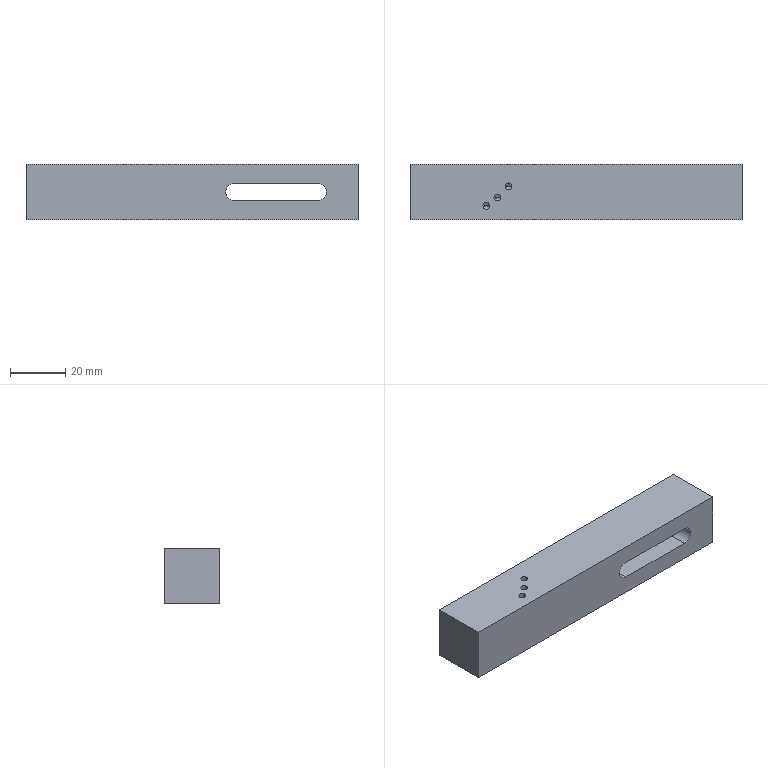Part | SolidWorks | features ICE 5, HoleWzd 2, Extrusion 1 | 1 solid | 22 faces | box 120 x 20 x 20 mm | volume 43402 mm3 | cylinder 8 | plane 8 | cone 6 | commonest cylinder face diameters 2.5 x6 6.4 x2
STEP:
#1=CARTESIAN_POINT('',(-64.65,108.,2.5));
#2=VERTEX_POINT('',#1);
#3=CARTESIAN_POINT('',(-62.15,108.,2.5));
#4=VERTEX_POINT('',#3);
#5=CARTESIAN_POINT('',(-63.4,108.,2.5));
#6=DIRECTION('',(0.,0.,1.));
#7=DIRECTION('',(1.,0.,0.));
#8=AXIS2_PLACEMENT_3D('',#5,#6,#7);
#9=CIRCLE('',#8,1.25);
#10=EDGE_CURVE('',#2,#4,#9,.T.);
#11=ORIENTED_EDGE('',*,*,#10,.F.);
#12=CARTESIAN_POINT('',(-64.65,108.,10.));
#13=VERTEX_POINT('',#12);
#14=CARTESIAN_POINT('',(-64.65,108.,10.));
#15=DIRECTION('',(0.,0.,1.));
#16=VECTOR('',#15,1000.);
#17=LINE('',#14,#16);
#18=EDGE_CURVE('',#2,#13,#17,.T.);
#19=ORIENTED_EDGE('',*,*,#18,.T.);
#20=CARTESIAN_POINT('',(-62.15,108.,10.));
#21=VERTEX_POINT('',#20);
#22=CARTESIAN_POINT('',(-63.4,108.,10.));
#23=DIRECTION('',(0.,0.,1.));
#24=DIRECTION('',(1.,0.,0.));
#25=AXIS2_PLACEMENT_3D('',#22,#23,#24);
#26=CIRCLE('',#25,1.25);
#27=EDGE_CURVE('',#13,#21,#26,.T.);
#28=ORIENTED_EDGE('',*,*,#27,.T.);
#29=CARTESIAN_POINT('',(-62.15,108.,10.));
#30=DIRECTION('',(0.,0.,1.));
#31=VECTOR('',#30,1000.);
#32=LINE('',#29,#31);
#33=EDGE_CURVE('',#4,#21,#32,.T.);
#34=ORIENTED_EDGE('',*,*,#33,.F.);
#35=EDGE_LOOP('',(#11,#19,#28,#34));
#36=FACE_OUTER_BOUND('',#35,.T.);
#37=CARTESIAN_POINT('',(-63.4,108.,10.));
#38=DIRECTION('',(0.,0.,1.));
#39=DIRECTION('',(1.,0.,0.));
#40=AXIS2_PLACEMENT_3D('',#37,#38,#39);
#41=CYLINDRICAL_SURFACE('',#40,1.25);
#42=ADVANCED_FACE('',(#36),#41,.F.);
#43=CARTESIAN_POINT('',(-63.4,108.,1.749));
#44=VERTEX_POINT('',#43);
#45=CARTESIAN_POINT('',(-62.15,108.,2.5));
#46=DIRECTION('',(0.8572,0.,0.515));
#47=VECTOR('',#46,1000.);
#48=LINE('',#45,#47);
#49=EDGE_CURVE('',#44,#4,#48,.T.);
#50=ORIENTED_EDGE('',*,*,#49,.F.);
#51=CARTESIAN_POINT('',(-64.65,108.,2.5));
#52=DIRECTION('',(-0.8572,0.,0.515));
#53=VECTOR('',#52,1000.);
#54=LINE('',#51,#53);
#55=EDGE_CURVE('',#44,#2,#54,.T.);
#56=ORIENTED_EDGE('',*,*,#55,.T.);
#57=ORIENTED_EDGE('',*,*,#10,.T.);
#58=EDGE_LOOP('',(#50,#56,#57));
#59=FACE_OUTER_BOUND('',#58,.T.);
#60=CARTESIAN_POINT('',(-63.4,108.,2.5));
#61=DIRECTION('',(0.,0.,1.));
#62=DIRECTION('',(1.,0.,0.));
#63=AXIS2_PLACEMENT_3D('',#60,#61,#62);
#64=CONICAL_SURFACE('',#63,1.25,1.03);
#65=ADVANCED_FACE('',(#59),#64,.F.);
#66=CARTESIAN_POINT('',(-60.65,112.,2.5));
#67=VERTEX_POINT('',#66);
#68=CARTESIAN_POINT('',(-58.15,112.,2.5));
#69=VERTEX_POINT('',#68);
#70=CARTESIAN_POINT('',(-59.4,112.,2.5));
#71=DIRECTION('',(0.,0.,1.));
#72=DIRECTION('',(1.,0.,0.));
#73=AXIS2_PLACEMENT_3D('',#70,#71,#72);
#74=CIRCLE('',#73,1.25);
#75=EDGE_CURVE('',#67,#69,#74,.T.);
#76=ORIENTED_EDGE('',*,*,#75,.F.);
#77=CARTESIAN_POINT('',(-60.65,112.,10.));
#78=VERTEX_POINT('',#77);
#79=CARTESIAN_POINT('',(-60.65,112.,10.));
#80=DIRECTION('',(0.,0.,1.));
#81=VECTOR('',#80,1000.);
#82=LINE('',#79,#81);
#83=EDGE_CURVE('',#67,#78,#82,.T.);
#84=ORIENTED_EDGE('',*,*,#83,.T.);
#85=CARTESIAN_POINT('',(-58.15,112.,10.));
#86=VERTEX_POINT('',#85);
#87=CARTESIAN_POINT('',(-59.4,112.,10.));
#88=DIRECTION('',(0.,0.,1.));
#89=DIRECTION('',(1.,0.,0.));
#90=AXIS2_PLACEMENT_3D('',#87,#88,#89);
#91=CIRCLE('',#90,1.25);
#92=EDGE_CURVE('',#78,#86,#91,.T.);
#93=ORIENTED_EDGE('',*,*,#92,.T.);
#94=CARTESIAN_POINT('',(-58.15,112.,10.));
#95=DIRECTION('',(0.,0.,1.));
#96=VECTOR('',#95,1000.);
#97=LINE('',#94,#96);
#98=EDGE_CURVE('',#69,#86,#97,.T.);
#99=ORIENTED_EDGE('',*,*,#98,.F.);
#100=EDGE_LOOP('',(#76,#84,#93,#99));
#101=FACE_OUTER_BOUND('',#100,.T.);
#102=CARTESIAN_POINT('',(-59.4,112.,10.));
#103=DIRECTION('',(0.,0.,1.));
#104=DIRECTION('',(1.,0.,0.));
#105=AXIS2_PLACEMENT_3D('',#102,#103,#104);
#106=CYLINDRICAL_SURFACE('',#105,1.25);
#107=ADVANCED_FACE('',(#101),#106,.F.);
#108=CARTESIAN_POINT('',(-59.4,112.,1.749));
#109=VERTEX_POINT('',#108);
#110=CARTESIAN_POINT('',(-58.15,112.,2.5));
#111=DIRECTION('',(0.8572,0.,0.515));
#112=VECTOR('',#111,1000.);
#113=LINE('',#110,#112);
#114=EDGE_CURVE('',#109,#69,#113,.T.);
#115=ORIENTED_EDGE('',*,*,#114,.F.);
#116=CARTESIAN_POINT('',(-60.65,112.,2.5));
#117=DIRECTION('',(-0.8572,0.,0.515));
#118=VECTOR('',#117,1000.);
#119=LINE('',#116,#118);
#120=EDGE_CURVE('',#109,#67,#119,.T.);
#121=ORIENTED_EDGE('',*,*,#120,.T.);
#122=ORIENTED_EDGE('',*,*,#75,.T.);
#123=EDGE_LOOP('',(#115,#121,#122));
#124=FACE_OUTER_BOUND('',#123,.T.);
#125=CARTESIAN_POINT('',(-59.4,112.,2.5));
#126=DIRECTION('',(0.,0.,1.));
#127=DIRECTION('',(1.,0.,0.));
#128=AXIS2_PLACEMENT_3D('',#125,#126,#127);
#129=CONICAL_SURFACE('',#128,1.25,1.03);
#130=ADVANCED_FACE('',(#124),#129,.F.);
#131=CARTESIAN_POINT('',(-68.65,105.,2.5));
#132=VERTEX_POINT('',#131);
#133=CARTESIAN_POINT('',(-66.15,105.,2.5));
#134=VERTEX_POINT('',#133);
#135=CARTESIAN_POINT('',(-67.4,105.,2.5));
#136=DIRECTION('',(0.,0.,1.));
#137=DIRECTION('',(1.,0.,0.));
#138=AXIS2_PLACEMENT_3D('',#135,#136,#137);
#139=CIRCLE('',#138,1.25);
#140=EDGE_CURVE('',#132,#134,#139,.T.);
#141=ORIENTED_EDGE('',*,*,#140,.F.);
#142=CARTESIAN_POINT('',(-68.65,105.,10.));
#143=VERTEX_POINT('',#142);
#144=CARTESIAN_POINT('',(-68.65,105.,10.));
#145=DIRECTION('',(0.,0.,1.));
#146=VECTOR('',#145,1000.);
#147=LINE('',#144,#146);
#148=EDGE_CURVE('',#132,#143,#147,.T.);
#149=ORIENTED_EDGE('',*,*,#148,.T.);
#150=CARTESIAN_POINT('',(-66.15,105.,10.));
#151=VERTEX_POINT('',#150);
#152=CARTESIAN_POINT('',(-67.4,105.,10.));
#153=DIRECTION('',(0.,0.,1.));
#154=DIRECTION('',(1.,0.,0.));
#155=AXIS2_PLACEMENT_3D('',#152,#153,#154);
#156=CIRCLE('',#155,1.25);
#157=EDGE_CURVE('',#143,#151,#156,.T.);
#158=ORIENTED_EDGE('',*,*,#157,.T.);
#159=CARTESIAN_POINT('',(-66.15,105.,10.));
#160=DIRECTION('',(0.,0.,1.));
#161=VECTOR('',#160,1000.);
#162=LINE('',#159,#161);
#163=EDGE_CURVE('',#134,#151,#162,.T.);
#164=ORIENTED_EDGE('',*,*,#163,.F.);
#165=EDGE_LOOP('',(#141,#149,#158,#164));
#166=FACE_OUTER_BOUND('',#165,.T.);
#167=CARTESIAN_POINT('',(-67.4,105.,10.));
#168=DIRECTION('',(0.,0.,1.));
#169=DIRECTION('',(1.,0.,0.));
#170=AXIS2_PLACEMENT_3D('',#167,#168,#169);
#171=CYLINDRICAL_SURFACE('',#170,1.25);
#172=ADVANCED_FACE('',(#166),#171,.F.);
#173=CARTESIAN_POINT('',(-67.4,105.,1.749));
#174=VERTEX_POINT('',#173);
#175=CARTESIAN_POINT('',(-66.15,105.,2.5));
#176=DIRECTION('',(0.8572,0.,0.515));
#177=VECTOR('',#176,1000.);
#178=LINE('',#175,#177);
#179=EDGE_CURVE('',#174,#134,#178,.T.);
#180=ORIENTED_EDGE('',*,*,#179,.F.);
#181=CARTESIAN_POINT('',(-68.65,105.,2.5));
#182=DIRECTION('',(-0.8572,0.,0.515));
#183=VECTOR('',#182,1000.);
#184=LINE('',#181,#183);
#185=EDGE_CURVE('',#174,#132,#184,.T.);
#186=ORIENTED_EDGE('',*,*,#185,.T.);
#187=ORIENTED_EDGE('',*,*,#140,.T.);
#188=EDGE_LOOP('',(#180,#186,#187));
#189=FACE_OUTER_BOUND('',#188,.T.);
#190=CARTESIAN_POINT('',(-67.4,105.,2.5));
#191=DIRECTION('',(0.,0.,1.));
#192=DIRECTION('',(1.,0.,0.));
#193=AXIS2_PLACEMENT_3D('',#190,#191,#192);
#194=CONICAL_SURFACE('',#193,1.25,1.03);
#195=ADVANCED_FACE('',(#189),#194,.F.);
#196=CARTESIAN_POINT('',(25.,120.,-10.));
#197=VERTEX_POINT('',#196);
#198=CARTESIAN_POINT('',(25.,100.,-10.));
#199=VERTEX_POINT('',#198);
#200=CARTESIAN_POINT('',(25.,100.,-10.));
#201=DIRECTION('',(0.,-1.,0.));
#202=VECTOR('',#201,1000.);
#203=LINE('',#200,#202);
#204=EDGE_CURVE('',#197,#199,#203,.T.);
#205=ORIENTED_EDGE('',*,*,#204,.F.);
#206=CARTESIAN_POINT('',(25.,120.,10.));
#207=VERTEX_POINT('',#206);
#208=CARTESIAN_POINT('',(25.,120.,-10.));
#209=DIRECTION('',(0.,0.,1.));
#210=VECTOR('',#209,1000.);
#211=LINE('',#208,#210);
#212=EDGE_CURVE('',#197,#207,#211,.T.);
#213=ORIENTED_EDGE('',*,*,#212,.T.);
#214=CARTESIAN_POINT('',(25.,100.,10.));
#215=VERTEX_POINT('',#214);
#216=CARTESIAN_POINT('',(25.,100.,10.));
#217=DIRECTION('',(0.,-1.,0.));
#218=VECTOR('',#217,1000.);
#219=LINE('',#216,#218);
#220=EDGE_CURVE('',#207,#215,#219,.T.);
#221=ORIENTED_EDGE('',*,*,#220,.T.);
#222=CARTESIAN_POINT('',(25.,100.,10.));
#223=DIRECTION('',(0.,0.,-1.));
#224=VECTOR('',#223,1000.);
#225=LINE('',#222,#224);
#226=EDGE_CURVE('',#215,#199,#225,.T.);
#227=ORIENTED_EDGE('',*,*,#226,.T.);
#228=EDGE_LOOP('',(#205,#213,#221,#227));
#229=FACE_OUTER_BOUND('',#228,.T.);
#230=CARTESIAN_POINT('',(25.,100.,10.));
#231=DIRECTION('',(-1.,0.,0.));
#232=DIRECTION('',(0.,0.,1.));
#233=AXIS2_PLACEMENT_3D('',#230,#231,#232);
#234=PLANE('',#233);
#235=ADVANCED_FACE('',(#229),#234,.F.);
#236=CARTESIAN_POINT('',(-95.,100.,-10.));
#237=VERTEX_POINT('',#236);
#238=CARTESIAN_POINT('',(-95.,120.,-10.));
#239=VERTEX_POINT('',#238);
#240=CARTESIAN_POINT('',(-95.,100.,-10.));
#241=DIRECTION('',(0.,1.,0.));
#242=VECTOR('',#241,1000.);
#243=LINE('',#240,#242);
#244=EDGE_CURVE('',#237,#239,#243,.T.);
#245=ORIENTED_EDGE('',*,*,#244,.T.);
#246=CARTESIAN_POINT('',(-95.,120.,-10.));
#247=DIRECTION('',(1.,0.,0.));
#248=VECTOR('',#247,1000.);
#249=LINE('',#246,#248);
#250=EDGE_CURVE('',#239,#197,#249,.T.);
#251=ORIENTED_EDGE('',*,*,#250,.T.);
#252=ORIENTED_EDGE('',*,*,#204,.T.);
#253=CARTESIAN_POINT('',(-95.,100.,-10.));
#254=DIRECTION('',(1.,0.,0.));
#255=VECTOR('',#254,1000.);
#256=LINE('',#253,#255);
#257=EDGE_CURVE('',#237,#199,#256,.T.);
#258=ORIENTED_EDGE('',*,*,#257,.F.);
#259=EDGE_LOOP('',(#245,#251,#252,#258));
#260=FACE_OUTER_BOUND('',#259,.T.);
#261=CARTESIAN_POINT('',(-25.,100.,-10.));
#262=DIRECTION('',(0.,0.,1.));
#263=DIRECTION('',(1.,0.,0.));
#264=AXIS2_PLACEMENT_3D('',#261,#262,#263);
#265=PLANE('',#264);
#266=ADVANCED_FACE('',(#260),#265,.F.);
#267=CARTESIAN_POINT('',(-63.4,108.,10.));
#268=DIRECTION('',(0.,0.,1.));
#269=DIRECTION('',(1.,0.,0.));
#270=AXIS2_PLACEMENT_3D('',#267,#268,#269);
#271=CIRCLE('',#270,1.25);
#272=EDGE_CURVE('',#21,#13,#271,.T.);
#273=ORIENTED_EDGE('',*,*,#272,.F.);
#274=ORIENTED_EDGE('',*,*,#27,.F.);
#275=EDGE_LOOP('',(#273,#274));
#276=FACE_BOUND('',#275,.T.);
#277=CARTESIAN_POINT('',(-59.4,112.,10.));
#278=DIRECTION('',(0.,0.,1.));
#279=DIRECTION('',(1.,0.,0.));
#280=AXIS2_PLACEMENT_3D('',#277,#278,#279);
#281=CIRCLE('',#280,1.25);
#282=EDGE_CURVE('',#86,#78,#281,.T.);
#283=ORIENTED_EDGE('',*,*,#282,.F.);
#284=ORIENTED_EDGE('',*,*,#92,.F.);
#285=EDGE_LOOP('',(#283,#284));
#286=FACE_BOUND('',#285,.T.);
#287=CARTESIAN_POINT('',(-67.4,105.,10.));
#288=DIRECTION('',(0.,0.,1.));
#289=DIRECTION('',(1.,0.,0.));
#290=AXIS2_PLACEMENT_3D('',#287,#288,#289);
#291=CIRCLE('',#290,1.25);
#292=EDGE_CURVE('',#151,#143,#291,.T.);
#293=ORIENTED_EDGE('',*,*,#292,.F.);
#294=ORIENTED_EDGE('',*,*,#157,.F.);
#295=EDGE_LOOP('',(#293,#294));
#296=FACE_BOUND('',#295,.T.);
#297=ORIENTED_EDGE('',*,*,#220,.F.);
#298=CARTESIAN_POINT('',(-95.,120.,10.));
#299=VERTEX_POINT('',#298);
#300=CARTESIAN_POINT('',(-95.,120.,10.));
#301=DIRECTION('',(1.,0.,0.));
#302=VECTOR('',#301,1000.);
#303=LINE('',#300,#302);
#304=EDGE_CURVE('',#299,#207,#303,.T.);
#305=ORIENTED_EDGE('',*,*,#304,.F.);
#306=CARTESIAN_POINT('',(-95.,100.,10.));
#307=VERTEX_POINT('',#306);
#308=CARTESIAN_POINT('',(-95.,100.,10.));
#309=DIRECTION('',(0.,-1.,0.));
#310=VECTOR('',#309,1000.);
#311=LINE('',#308,#310);
#312=EDGE_CURVE('',#299,#307,#311,.T.);
#313=ORIENTED_EDGE('',*,*,#312,.T.);
#314=CARTESIAN_POINT('',(-95.,100.,10.));
#315=DIRECTION('',(1.,0.,0.));
#316=VECTOR('',#315,1000.);
#317=LINE('',#314,#316);
#318=EDGE_CURVE('',#307,#215,#317,.T.);
#319=ORIENTED_EDGE('',*,*,#318,.T.);
#320=EDGE_LOOP('',(#297,#305,#313,#319));
#321=FACE_OUTER_BOUND('',#320,.T.);
#322=CARTESIAN_POINT('',(-25.,100.,10.));
#323=DIRECTION('',(0.,0.,-1.));
#324=DIRECTION('',(-1.,0.,0.));
#325=AXIS2_PLACEMENT_3D('',#322,#323,#324);
#326=PLANE('',#325);
#327=ADVANCED_FACE('',(#276,#286,#296,#321),#326,.F.);
#328=CARTESIAN_POINT('',(10.388,100.,3.2));
#329=VERTEX_POINT('',#328);
#330=CARTESIAN_POINT('',(10.388,100.,-3.2));
#331=VERTEX_POINT('',#330);
#332=CARTESIAN_POINT('',(10.388,100.,0.));
#333=DIRECTION('',(0.,1.,0.));
#334=DIRECTION('',(0.,0.,1.));
#335=AXIS2_PLACEMENT_3D('',#332,#333,#334);
#336=CIRCLE('',#335,3.2);
#337=EDGE_CURVE('',#329,#331,#336,.T.);
#338=ORIENTED_EDGE('',*,*,#337,.T.);
#339=CARTESIAN_POINT('',(-19.612,100.,-3.2));
#340=VERTEX_POINT('',#339);
#341=CARTESIAN_POINT('',(10.388,100.,-3.2));
#342=DIRECTION('',(-1.,0.,0.));
#343=VECTOR('',#342,1000.);
#344=LINE('',#341,#343);
#345=EDGE_CURVE('',#331,#340,#344,.T.);
#346=ORIENTED_EDGE('',*,*,#345,.T.);
#347=CARTESIAN_POINT('',(-19.612,100.,3.2));
#348=VERTEX_POINT('',#347);
#349=CARTESIAN_POINT('',(-19.612,100.,0.));
#350=DIRECTION('',(0.,1.,0.));
#351=DIRECTION('',(0.,0.,1.));
#352=AXIS2_PLACEMENT_3D('',#349,#350,#351);
#353=CIRCLE('',#352,3.2);
#354=EDGE_CURVE('',#340,#348,#353,.T.);
#355=ORIENTED_EDGE('',*,*,#354,.T.);
#356=CARTESIAN_POINT('',(10.388,100.,3.2));
#357=DIRECTION('',(1.,0.,0.));
#358=VECTOR('',#357,1000.);
#359=LINE('',#356,#358);
#360=EDGE_CURVE('',#348,#329,#359,.T.);
#361=ORIENTED_EDGE('',*,*,#360,.T.);
#362=EDGE_LOOP('',(#338,#346,#355,#361));
#363=FACE_BOUND('',#362,.T.);
#364=ORIENTED_EDGE('',*,*,#257,.T.);
#365=ORIENTED_EDGE('',*,*,#226,.F.);
#366=ORIENTED_EDGE('',*,*,#318,.F.);
#367=CARTESIAN_POINT('',(-95.,100.,-10.));
#368=DIRECTION('',(0.,0.,-1.));
#369=VECTOR('',#368,1000.);
#370=LINE('',#367,#369);
#371=EDGE_CURVE('',#307,#237,#370,.T.);
#372=ORIENTED_EDGE('',*,*,#371,.T.);
#373=EDGE_LOOP('',(#364,#365,#366,#372));
#374=FACE_OUTER_BOUND('',#373,.T.);
#375=CARTESIAN_POINT('',(-95.,100.,-10.));
#376=DIRECTION('',(0.,-1.,0.));
#377=DIRECTION('',(0.,0.,-1.));
#378=AXIS2_PLACEMENT_3D('',#375,#376,#377);
#379=PLANE('',#378);
#380=ADVANCED_FACE('',(#363,#374),#379,.T.);
#381=ORIENTED_EDGE('',*,*,#312,.F.);
#382=CARTESIAN_POINT('',(-95.,120.,-10.));
#383=DIRECTION('',(0.,0.,1.));
#384=VECTOR('',#383,1000.);
#385=LINE('',#382,#384);
#386=EDGE_CURVE('',#239,#299,#385,.T.);
#387=ORIENTED_EDGE('',*,*,#386,.F.);
#388=ORIENTED_EDGE('',*,*,#244,.F.);
#389=ORIENTED_EDGE('',*,*,#371,.F.);
#390=EDGE_LOOP('',(#381,#387,#388,#389));
#391=FACE_OUTER_BOUND('',#390,.T.);
#392=CARTESIAN_POINT('',(-95.,0.,0.));
#393=DIRECTION('',(1.,0.,0.));
#394=DIRECTION('',(0.,0.,-1.));
#395=AXIS2_PLACEMENT_3D('',#392,#393,#394);
#396=PLANE('',#395);
#397=ADVANCED_FACE('',(#391),#396,.F.);
#398=ORIENTED_EDGE('',*,*,#185,.F.);
#399=ORIENTED_EDGE('',*,*,#179,.T.);
#400=CARTESIAN_POINT('',(-67.4,105.,2.5));
#401=DIRECTION('',(0.,0.,1.));
#402=DIRECTION('',(1.,0.,0.));
#403=AXIS2_PLACEMENT_3D('',#400,#401,#402);
#404=CIRCLE('',#403,1.25);
#405=EDGE_CURVE('',#134,#132,#404,.T.);
#406=ORIENTED_EDGE('',*,*,#405,.T.);
#407=EDGE_LOOP('',(#398,#399,#406));
#408=FACE_OUTER_BOUND('',#407,.T.);
#409=CARTESIAN_POINT('',(-67.4,105.,2.5));
#410=DIRECTION('',(0.,0.,1.));
#411=DIRECTION('',(1.,0.,0.));
#412=AXIS2_PLACEMENT_3D('',#409,#410,#411);
#413=CONICAL_SURFACE('',#412,1.25,1.03);
#414=ADVANCED_FACE('',(#408),#413,.F.);
#415=ORIENTED_EDGE('',*,*,#148,.F.);
#416=ORIENTED_EDGE('',*,*,#405,.F.);
#417=ORIENTED_EDGE('',*,*,#163,.T.);
#418=ORIENTED_EDGE('',*,*,#292,.T.);
#419=EDGE_LOOP('',(#415,#416,#417,#418));
#420=FACE_OUTER_BOUND('',#419,.T.);
#421=CARTESIAN_POINT('',(-67.4,105.,10.));
#422=DIRECTION('',(0.,0.,1.));
#423=DIRECTION('',(1.,0.,0.));
#424=AXIS2_PLACEMENT_3D('',#421,#422,#423);
#425=CYLINDRICAL_SURFACE('',#424,1.25);
#426=ADVANCED_FACE('',(#420),#425,.F.);
#427=ORIENTED_EDGE('',*,*,#120,.F.);
#428=ORIENTED_EDGE('',*,*,#114,.T.);
#429=CARTESIAN_POINT('',(-59.4,112.,2.5));
#430=DIRECTION('',(0.,0.,1.));
#431=DIRECTION('',(1.,0.,0.));
#432=AXIS2_PLACEMENT_3D('',#429,#430,#431);
#433=CIRCLE('',#432,1.25);
#434=EDGE_CURVE('',#69,#67,#433,.T.);
#435=ORIENTED_EDGE('',*,*,#434,.T.);
#436=EDGE_LOOP('',(#427,#428,#435));
#437=FACE_OUTER_BOUND('',#436,.T.);
#438=CARTESIAN_POINT('',(-59.4,112.,2.5));
#439=DIRECTION('',(0.,0.,1.));
#440=DIRECTION('',(1.,0.,0.));
#441=AXIS2_PLACEMENT_3D('',#438,#439,#440);
#442=CONICAL_SURFACE('',#441,1.25,1.03);
#443=ADVANCED_FACE('',(#437),#442,.F.);
#444=ORIENTED_EDGE('',*,*,#83,.F.);
#445=ORIENTED_EDGE('',*,*,#434,.F.);
#446=ORIENTED_EDGE('',*,*,#98,.T.);
#447=ORIENTED_EDGE('',*,*,#282,.T.);
#448=EDGE_LOOP('',(#444,#445,#446,#447));
#449=FACE_OUTER_BOUND('',#448,.T.);
#450=CARTESIAN_POINT('',(-59.4,112.,10.));
#451=DIRECTION('',(0.,0.,1.));
#452=DIRECTION('',(1.,0.,0.));
#453=AXIS2_PLACEMENT_3D('',#450,#451,#452);
#454=CYLINDRICAL_SURFACE('',#453,1.25);
#455=ADVANCED_FACE('',(#449),#454,.F.);
#456=ORIENTED_EDGE('',*,*,#55,.F.);
#457=ORIENTED_EDGE('',*,*,#49,.T.);
#458=CARTESIAN_POINT('',(-63.4,108.,2.5));
#459=DIRECTION('',(0.,0.,1.));
#460=DIRECTION('',(1.,0.,0.));
#461=AXIS2_PLACEMENT_3D('',#458,#459,#460);
#462=CIRCLE('',#461,1.25);
#463=EDGE_CURVE('',#4,#2,#462,.T.);
#464=ORIENTED_EDGE('',*,*,#463,.T.);
#465=EDGE_LOOP('',(#456,#457,#464));
#466=FACE_OUTER_BOUND('',#465,.T.);
#467=CARTESIAN_POINT('',(-63.4,108.,2.5));
#468=DIRECTION('',(0.,0.,1.));
#469=DIRECTION('',(1.,0.,0.));
#470=AXIS2_PLACEMENT_3D('',#467,#468,#469);
#471=CONICAL_SURFACE('',#470,1.25,1.03);
#472=ADVANCED_FACE('',(#466),#471,.F.);
#473=ORIENTED_EDGE('',*,*,#18,.F.);
#474=ORIENTED_EDGE('',*,*,#463,.F.);
#475=ORIENTED_EDGE('',*,*,#33,.T.);
#476=ORIENTED_EDGE('',*,*,#272,.T.);
#477=EDGE_LOOP('',(#473,#474,#475,#476));
#478=FACE_OUTER_BOUND('',#477,.T.);
#479=CARTESIAN_POINT('',(-63.4,108.,10.));
#480=DIRECTION('',(0.,0.,1.));
#481=DIRECTION('',(1.,0.,0.));
#482=AXIS2_PLACEMENT_3D('',#479,#480,#481);
#483=CYLINDRICAL_SURFACE('',#482,1.25);
#484=ADVANCED_FACE('',(#478),#483,.F.);
#485=CARTESIAN_POINT('',(10.388,120.,3.2));
#486=VERTEX_POINT('',#485);
#487=CARTESIAN_POINT('',(10.388,100.,3.2));
#488=DIRECTION('',(0.,1.,0.));
#489=VECTOR('',#488,1000.);
#490=LINE('',#487,#489);
#491=EDGE_CURVE('',#329,#486,#490,.T.);
#492=ORIENTED_EDGE('',*,*,#491,.T.);
#493=CARTESIAN_POINT('',(10.388,120.,-3.2));
#494=VERTEX_POINT('',#493);
#495=CARTESIAN_POINT('',(10.388,120.,0.));
#496=DIRECTION('',(0.,1.,0.));
#497=DIRECTION('',(0.,0.,-1.));
#498=AXIS2_PLACEMENT_3D('',#495,#496,#497);
#499=CIRCLE('',#498,3.2);
#500=EDGE_CURVE('',#486,#494,#499,.T.);
#501=ORIENTED_EDGE('',*,*,#500,.T.);
#502=CARTESIAN_POINT('',(10.388,100.,-3.2));
#503=DIRECTION('',(0.,1.,0.));
#504=VECTOR('',#503,1000.);
#505=LINE('',#502,#504);
#506=EDGE_CURVE('',#331,#494,#505,.T.);
#507=ORIENTED_EDGE('',*,*,#506,.F.);
#508=ORIENTED_EDGE('',*,*,#337,.F.);
#509=EDGE_LOOP('',(#492,#501,#507,#508));
#510=FACE_OUTER_BOUND('',#509,.T.);
#511=CARTESIAN_POINT('',(10.388,100.,0.));
#512=DIRECTION('',(0.,1.,0.));
#513=DIRECTION('',(0.,0.,1.));
#514=AXIS2_PLACEMENT_3D('',#511,#512,#513);
#515=CYLINDRICAL_SURFACE('',#514,3.2);
#516=ADVANCED_FACE('',(#510),#515,.F.);
#517=CARTESIAN_POINT('',(-19.612,120.,3.2));
#518=VERTEX_POINT('',#517);
#519=CARTESIAN_POINT('',(-19.612,100.,3.2));
#520=DIRECTION('',(0.,1.,0.));
#521=VECTOR('',#520,1000.);
#522=LINE('',#519,#521);
#523=EDGE_CURVE('',#348,#518,#522,.T.);
#524=ORIENTED_EDGE('',*,*,#523,.T.);
#525=CARTESIAN_POINT('',(10.388,120.,3.2));
#526=DIRECTION('',(1.,0.,0.));
#527=VECTOR('',#526,1000.);
#528=LINE('',#525,#527);
#529=EDGE_CURVE('',#518,#486,#528,.T.);
#530=ORIENTED_EDGE('',*,*,#529,.T.);
#531=ORIENTED_EDGE('',*,*,#491,.F.);
#532=ORIENTED_EDGE('',*,*,#360,.F.);
#533=EDGE_LOOP('',(#524,#530,#531,#532));
#534=FACE_OUTER_BOUND('',#533,.T.);
#535=CARTESIAN_POINT('',(10.388,100.,3.2));
#536=DIRECTION('',(0.,0.,1.));
#537=DIRECTION('',(1.,0.,0.));
#538=AXIS2_PLACEMENT_3D('',#535,#536,#537);
#539=PLANE('',#538);
#540=ADVANCED_FACE('',(#534),#539,.F.);
#541=CARTESIAN_POINT('',(-19.612,120.,-3.2));
#542=VERTEX_POINT('',#541);
#543=CARTESIAN_POINT('',(-19.612,100.,-3.2));
#544=DIRECTION('',(0.,1.,0.));
#545=VECTOR('',#544,1000.);
#546=LINE('',#543,#545);
#547=EDGE_CURVE('',#340,#542,#546,.T.);
#548=ORIENTED_EDGE('',*,*,#547,.T.);
#549=CARTESIAN_POINT('',(-19.612,120.,0.));
#550=DIRECTION('',(0.,1.,0.));
#551=DIRECTION('',(0.,0.,-1.));
#552=AXIS2_PLACEMENT_3D('',#549,#550,#551);
#553=CIRCLE('',#552,3.2);
#554=EDGE_CURVE('',#542,#518,#553,.T.);
#555=ORIENTED_EDGE('',*,*,#554,.T.);
#556=ORIENTED_EDGE('',*,*,#523,.F.);
#557=ORIENTED_EDGE('',*,*,#354,.F.);
#558=EDGE_LOOP('',(#548,#555,#556,#557));
#559=FACE_OUTER_BOUND('',#558,.T.);
#560=CARTESIAN_POINT('',(-19.612,100.,0.));
#561=DIRECTION('',(0.,1.,0.));
#562=DIRECTION('',(0.,0.,1.));
#563=AXIS2_PLACEMENT_3D('',#560,#561,#562);
#564=CYLINDRICAL_SURFACE('',#563,3.2);
#565=ADVANCED_FACE('',(#559),#564,.F.);
#566=ORIENTED_EDGE('',*,*,#506,.T.);
#567=CARTESIAN_POINT('',(10.388,120.,-3.2));
#568=DIRECTION('',(-1.,0.,0.));
#569=VECTOR('',#568,1000.);
#570=LINE('',#567,#569);
#571=EDGE_CURVE('',#494,#542,#570,.T.);
#572=ORIENTED_EDGE('',*,*,#571,.T.);
#573=ORIENTED_EDGE('',*,*,#547,.F.);
#574=ORIENTED_EDGE('',*,*,#345,.F.);
#575=EDGE_LOOP('',(#566,#572,#573,#574));
#576=FACE_OUTER_BOUND('',#575,.T.);
#577=CARTESIAN_POINT('',(10.388,100.,-3.2));
#578=DIRECTION('',(0.,0.,-1.));
#579=DIRECTION('',(-1.,0.,0.));
#580=AXIS2_PLACEMENT_3D('',#577,#578,#579);
#581=PLANE('',#580);
#582=ADVANCED_FACE('',(#576),#581,.F.);
#583=ORIENTED_EDGE('',*,*,#304,.T.);
#584=ORIENTED_EDGE('',*,*,#212,.F.);
#585=ORIENTED_EDGE('',*,*,#250,.F.);
#586=ORIENTED_EDGE('',*,*,#386,.T.);
#587=EDGE_LOOP('',(#583,#584,#585,#586));
#588=FACE_OUTER_BOUND('',#587,.T.);
#589=ORIENTED_EDGE('',*,*,#529,.F.);
#590=ORIENTED_EDGE('',*,*,#554,.F.);
#591=ORIENTED_EDGE('',*,*,#571,.F.);
#592=ORIENTED_EDGE('',*,*,#500,.F.);
#593=EDGE_LOOP('',(#589,#590,#591,#592));
#594=FACE_BOUND('',#593,.T.);
#595=CARTESIAN_POINT('',(-95.,120.,-10.));
#596=DIRECTION('',(0.,-1.,0.));
#597=DIRECTION('',(0.,0.,-1.));
#598=AXIS2_PLACEMENT_3D('',#595,#596,#597);
#599=PLANE('',#598);
#600=ADVANCED_FACE('',(#588,#594),#599,.F.);
#601=CLOSED_SHELL('',(#42,#65,#107,#130,#172,#195,#235,#266,#327,#380,#397,#414,#426,#443,#455,#472,#484,#516,#540,#565,#582,#600));
#602=MANIFOLD_SOLID_BREP('',#601);
#603=CARTESIAN_POINT('',(0.,0.,0.));
#604=DIRECTION('',(0.,0.,1.));
#605=DIRECTION('',(1.,0.,0.));
#606=AXIS2_PLACEMENT_3D('',#603,#604,#605);
#607=(LENGTH_UNIT()NAMED_UNIT(*)SI_UNIT(.MILLI.,.METRE.));
#608=UNCERTAINTY_MEASURE_WITH_UNIT(LENGTH_MEASURE(0.00001),#607,'','');
#609=(NAMED_UNIT(*)PLANE_ANGLE_UNIT()SI_UNIT($,.RADIAN.));
#610=(NAMED_UNIT(*)SI_UNIT($,.STERADIAN.)SOLID_ANGLE_UNIT());
#611=(GEOMETRIC_REPRESENTATION_CONTEXT(3)GLOBAL_UNCERTAINTY_ASSIGNED_CONTEXT((#608))GLOBAL_UNIT_ASSIGNED_CONTEXT((#607,#609,#610))REPRESENTATION_CONTEXT('',''));
#612=ADVANCED_BREP_SHAPE_REPRESENTATION('',(#602,#606),#611);